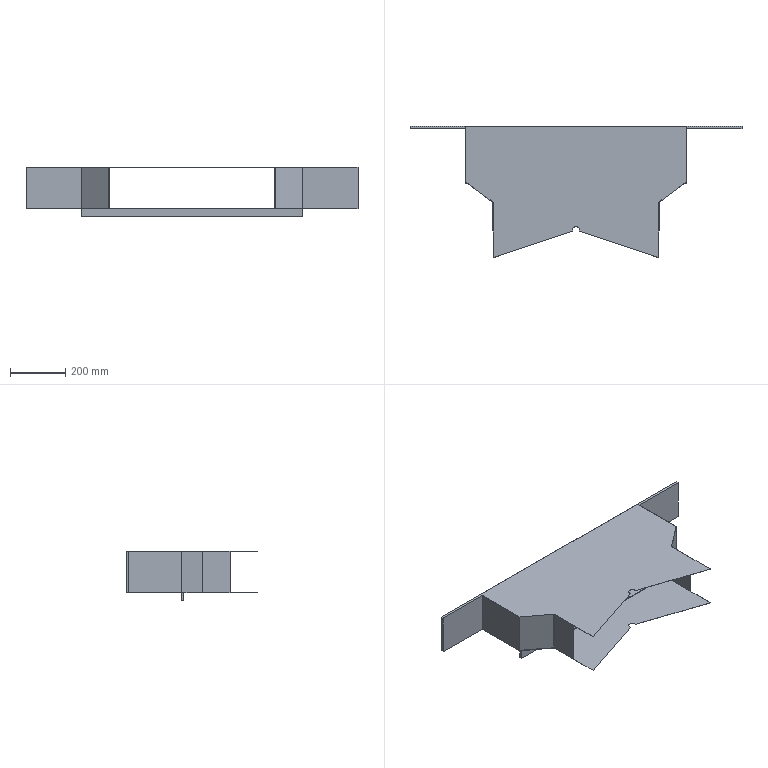Part | SolidWorks | features ICE 9, Extrusion 1 | 1 solid | 50 faces | box 1201 x 475 x 180 mm | volume 1092637 mm3 | plane 48 | cylinder 2 | commonest cylinder face diameters 25 x2
STEP:
#1=CARTESIAN_POINT('',(-399.925,274.7,0.));
#2=VERTEX_POINT('',#1);
#3=CARTESIAN_POINT('',(-399.598,274.7,0.));
#4=VERTEX_POINT('',#3);
#5=CARTESIAN_POINT('',(400.075,275.,0.));
#6=DIRECTION('',(1.,0.0003753,0.));
#7=VECTOR('',#6,1000.);
#8=LINE('',#5,#7);
#9=EDGE_CURVE('',#2,#4,#8,.T.);
#10=ORIENTED_EDGE('',*,*,#9,.F.);
#11=CARTESIAN_POINT('',(-399.925,274.195,0.));
#12=VERTEX_POINT('',#11);
#13=CARTESIAN_POINT('',(-399.922,266.7,0.));
#14=DIRECTION('',(-0.0003753,1.,0.));
#15=VECTOR('',#14,1000.);
#16=LINE('',#13,#15);
#17=EDGE_CURVE('',#12,#2,#16,.T.);
#18=ORIENTED_EDGE('',*,*,#17,.F.);
#19=CARTESIAN_POINT('',(-400.6,274.7,0.));
#20=VERTEX_POINT('',#19);
#21=CARTESIAN_POINT('',(-400.6,274.7,0.));
#22=DIRECTION('',(-0.8012,0.5985,0.));
#23=VECTOR('',#22,1000.);
#24=LINE('',#21,#23);
#25=EDGE_CURVE('',#12,#20,#24,.T.);
#26=ORIENTED_EDGE('',*,*,#25,.T.);
#27=CARTESIAN_POINT('',(-400.6,467.317,0.));
#28=VERTEX_POINT('',#27);
#29=CARTESIAN_POINT('',(-400.6,274.7,0.));
#30=DIRECTION('',(0.,1.,0.));
#31=VECTOR('',#30,1000.);
#32=LINE('',#29,#31);
#33=EDGE_CURVE('',#20,#28,#32,.T.);
#34=ORIENTED_EDGE('',*,*,#33,.T.);
#35=CARTESIAN_POINT('',(-600.6,467.317,0.));
#36=VERTEX_POINT('',#35);
#37=CARTESIAN_POINT('',(-600.6,467.317,0.));
#38=DIRECTION('',(1.,0.,0.));
#39=VECTOR('',#38,1000.);
#40=LINE('',#37,#39);
#41=EDGE_CURVE('',#36,#28,#40,.T.);
#42=ORIENTED_EDGE('',*,*,#41,.F.);
#43=CARTESIAN_POINT('',(-600.6,475.,0.));
#44=VERTEX_POINT('',#43);
#45=CARTESIAN_POINT('',(-600.6,467.317,0.));
#46=DIRECTION('',(0.,-1.,0.));
#47=VECTOR('',#46,1000.);
#48=LINE('',#45,#47);
#49=EDGE_CURVE('',#44,#36,#48,.T.);
#50=ORIENTED_EDGE('',*,*,#49,.F.);
#51=CARTESIAN_POINT('',(-400.,475.,0.));
#52=VERTEX_POINT('',#51);
#53=CARTESIAN_POINT('',(-400.6,475.,0.));
#54=DIRECTION('',(-1.,0.,0.));
#55=VECTOR('',#54,1000.);
#56=LINE('',#53,#55);
#57=EDGE_CURVE('',#52,#44,#56,.T.);
#58=ORIENTED_EDGE('',*,*,#57,.F.);
#59=CARTESIAN_POINT('',(-400.,275.,0.));
#60=VERTEX_POINT('',#59);
#61=CARTESIAN_POINT('',(-400.,375.,0.));
#62=DIRECTION('',(0.,-1.,0.));
#63=VECTOR('',#62,1000.);
#64=LINE('',#61,#63);
#65=EDGE_CURVE('',#52,#60,#64,.T.);
#66=ORIENTED_EDGE('',*,*,#65,.T.);
#67=CARTESIAN_POINT('',(-400.,275.,0.));
#68=DIRECTION('',(0.8012,-0.5985,0.));
#69=VECTOR('',#68,1000.);
#70=LINE('',#67,#69);
#71=EDGE_CURVE('',#60,#4,#70,.T.);
#72=ORIENTED_EDGE('',*,*,#71,.T.);
#73=EDGE_LOOP('',(#10,#18,#26,#34,#42,#50,#58,#66,#72));
#74=FACE_OUTER_BOUND('',#73,.T.);
#75=CARTESIAN_POINT('',(0.,100.,0.));
#76=DIRECTION('',(0.,0.,1.));
#77=DIRECTION('',(1.,0.,0.));
#78=AXIS2_PLACEMENT_3D('',#75,#76,#77);
#79=PLANE('',#78);
#80=ADVANCED_FACE('',(#74),#79,.F.);
#81=CARTESIAN_POINT('',(400.,275.,0.));
#82=VERTEX_POINT('',#81);
#83=CARTESIAN_POINT('',(400.075,275.,0.));
#84=VERTEX_POINT('',#83);
#85=CARTESIAN_POINT('',(400.075,275.,0.));
#86=DIRECTION('',(1.,0.0003753,0.));
#87=VECTOR('',#86,1000.);
#88=LINE('',#85,#87);
#89=EDGE_CURVE('',#82,#84,#88,.T.);
#90=ORIENTED_EDGE('',*,*,#89,.F.);
#91=CARTESIAN_POINT('',(400.,475.,0.));
#92=VERTEX_POINT('',#91);
#93=CARTESIAN_POINT('',(400.,375.,0.));
#94=DIRECTION('',(0.,1.,0.));
#95=VECTOR('',#94,1000.);
#96=LINE('',#93,#95);
#97=EDGE_CURVE('',#82,#92,#96,.T.);
#98=ORIENTED_EDGE('',*,*,#97,.T.);
#99=CARTESIAN_POINT('',(600.6,475.,0.));
#100=VERTEX_POINT('',#99);
#101=CARTESIAN_POINT('',(400.6,475.,0.));
#102=DIRECTION('',(-1.,0.,0.));
#103=VECTOR('',#102,1000.);
#104=LINE('',#101,#103);
#105=EDGE_CURVE('',#100,#92,#104,.T.);
#106=ORIENTED_EDGE('',*,*,#105,.F.);
#107=CARTESIAN_POINT('',(600.6,465.599,0.));
#108=VERTEX_POINT('',#107);
#109=CARTESIAN_POINT('',(600.6,475.,0.));
#110=DIRECTION('',(0.,1.,0.));
#111=VECTOR('',#110,1000.);
#112=LINE('',#109,#111);
#113=EDGE_CURVE('',#108,#100,#112,.T.);
#114=ORIENTED_EDGE('',*,*,#113,.F.);
#115=CARTESIAN_POINT('',(400.6,465.599,0.));
#116=VERTEX_POINT('',#115);
#117=CARTESIAN_POINT('',(600.6,465.599,0.));
#118=DIRECTION('',(-1.,0.,0.));
#119=VECTOR('',#118,1000.);
#120=LINE('',#117,#119);
#121=EDGE_CURVE('',#108,#116,#120,.T.);
#122=ORIENTED_EDGE('',*,*,#121,.T.);
#123=CARTESIAN_POINT('',(400.6,274.7,0.));
#124=VERTEX_POINT('',#123);
#125=CARTESIAN_POINT('',(400.6,274.7,0.));
#126=DIRECTION('',(0.,-1.,0.));
#127=VECTOR('',#126,1000.);
#128=LINE('',#125,#127);
#129=EDGE_CURVE('',#116,#124,#128,.T.);
#130=ORIENTED_EDGE('',*,*,#129,.T.);
#131=CARTESIAN_POINT('',(400.075,274.307,0.));
#132=VERTEX_POINT('',#131);
#133=CARTESIAN_POINT('',(400.6,274.7,0.));
#134=DIRECTION('',(-0.8012,-0.5985,0.));
#135=VECTOR('',#134,1000.);
#136=LINE('',#133,#135);
#137=EDGE_CURVE('',#124,#132,#136,.T.);
#138=ORIENTED_EDGE('',*,*,#137,.T.);
#139=CARTESIAN_POINT('',(400.078,267.,0.));
#140=DIRECTION('',(-0.0003753,1.,0.));
#141=VECTOR('',#140,1000.);
#142=LINE('',#139,#141);
#143=EDGE_CURVE('',#132,#84,#142,.T.);
#144=ORIENTED_EDGE('',*,*,#143,.T.);
#145=EDGE_LOOP('',(#90,#98,#106,#114,#122,#130,#138,#144));
#146=FACE_OUTER_BOUND('',#145,.T.);
#147=CARTESIAN_POINT('',(0.,100.,0.));
#148=DIRECTION('',(0.,0.,1.));
#149=DIRECTION('',(1.,0.,0.));
#150=AXIS2_PLACEMENT_3D('',#147,#148,#149);
#151=PLANE('',#150);
#152=ADVANCED_FACE('',(#146),#151,.F.);
#153=CARTESIAN_POINT('',(-300.,200.301,149.4));
#154=VERTEX_POINT('',#153);
#155=CARTESIAN_POINT('',(-300.,200.301,0.6));
#156=VERTEX_POINT('',#155);
#157=CARTESIAN_POINT('',(-300.,200.301,150.));
#158=DIRECTION('',(0.,0.,-1.));
#159=VECTOR('',#158,1000.);
#160=LINE('',#157,#159);
#161=EDGE_CURVE('',#154,#156,#160,.T.);
#162=ORIENTED_EDGE('',*,*,#161,.F.);
#163=CARTESIAN_POINT('',(-300.,100.,149.4));
#164=VERTEX_POINT('',#163);
#165=CARTESIAN_POINT('',(-300.,200.,149.4));
#166=DIRECTION('',(0.,-1.,0.));
#167=VECTOR('',#166,1000.);
#168=LINE('',#165,#167);
#169=EDGE_CURVE('',#154,#164,#168,.T.);
#170=ORIENTED_EDGE('',*,*,#169,.T.);
#171=CARTESIAN_POINT('',(-300.,100.,0.6));
#172=VERTEX_POINT('',#171);
#173=CARTESIAN_POINT('',(-300.,100.,150.));
#174=DIRECTION('',(0.,0.,-1.));
#175=VECTOR('',#174,1000.);
#176=LINE('',#173,#175);
#177=EDGE_CURVE('',#164,#172,#176,.T.);
#178=ORIENTED_EDGE('',*,*,#177,.T.);
#179=CARTESIAN_POINT('',(-300.,230.,0.6));
#180=DIRECTION('',(0.,-1.,0.));
#181=VECTOR('',#180,1000.);
#182=LINE('',#179,#181);
#183=EDGE_CURVE('',#156,#172,#182,.T.);
#184=ORIENTED_EDGE('',*,*,#183,.F.);
#185=EDGE_LOOP('',(#162,#170,#178,#184));
#186=FACE_OUTER_BOUND('',#185,.T.);
#187=CARTESIAN_POINT('',(-300.,200.,150.));
#188=DIRECTION('',(1.,0.,0.));
#189=DIRECTION('',(0.,0.,-1.));
#190=AXIS2_PLACEMENT_3D('',#187,#188,#189);
#191=PLANE('',#190);
#192=ADVANCED_FACE('',(#186),#191,.T.);
#193=CARTESIAN_POINT('',(-399.598,274.7,2.));
#194=VERTEX_POINT('',#193);
#195=CARTESIAN_POINT('',(-399.598,274.7,150.));
#196=DIRECTION('',(0.,0.,1.));
#197=VECTOR('',#196,1000.);
#198=LINE('',#195,#197);
#199=EDGE_CURVE('',#4,#194,#198,.T.);
#200=ORIENTED_EDGE('',*,*,#199,.F.);
#201=ORIENTED_EDGE('',*,*,#71,.F.);
#202=CARTESIAN_POINT('',(-400.,275.,149.4));
#203=VERTEX_POINT('',#202);
#204=CARTESIAN_POINT('',(-400.,275.,150.));
#205=DIRECTION('',(0.,0.,-1.));
#206=VECTOR('',#205,1000.);
#207=LINE('',#204,#206);
#208=EDGE_CURVE('',#203,#60,#207,.T.);
#209=ORIENTED_EDGE('',*,*,#208,.F.);
#210=CARTESIAN_POINT('',(-400.,275.,149.4));
#211=DIRECTION('',(0.8012,-0.5985,0.));
#212=VECTOR('',#211,1000.);
#213=LINE('',#210,#212);
#214=EDGE_CURVE('',#203,#154,#213,.T.);
#215=ORIENTED_EDGE('',*,*,#214,.T.);
#216=ORIENTED_EDGE('',*,*,#161,.T.);
#217=CARTESIAN_POINT('',(-342.578,232.106,0.6));
#218=VERTEX_POINT('',#217);
#219=CARTESIAN_POINT('',(-400.,275.,0.6));
#220=DIRECTION('',(0.8012,-0.5985,0.));
#221=VECTOR('',#220,1000.);
#222=LINE('',#219,#221);
#223=EDGE_CURVE('',#218,#156,#222,.T.);
#224=ORIENTED_EDGE('',*,*,#223,.F.);
#225=CARTESIAN_POINT('',(-342.578,232.106,2.));
#226=VERTEX_POINT('',#225);
#227=CARTESIAN_POINT('',(-342.578,232.106,2.));
#228=DIRECTION('',(0.,0.,-1.));
#229=VECTOR('',#228,1000.);
#230=LINE('',#227,#229);
#231=EDGE_CURVE('',#226,#218,#230,.T.);
#232=ORIENTED_EDGE('',*,*,#231,.F.);
#233=CARTESIAN_POINT('',(-400.,275.,2.));
#234=DIRECTION('',(0.8012,-0.5985,0.));
#235=VECTOR('',#234,1000.);
#236=LINE('',#233,#235);
#237=EDGE_CURVE('',#194,#226,#236,.T.);
#238=ORIENTED_EDGE('',*,*,#237,.F.);
#239=EDGE_LOOP('',(#200,#201,#209,#215,#216,#224,#232,#238));
#240=FACE_OUTER_BOUND('',#239,.T.);
#241=CARTESIAN_POINT('',(-400.,275.,150.));
#242=DIRECTION('',(0.5985,0.8012,0.));
#243=DIRECTION('',(-0.8012,0.5985,0.));
#244=AXIS2_PLACEMENT_3D('',#241,#242,#243);
#245=PLANE('',#244);
#246=ADVANCED_FACE('',(#240),#245,.T.);
#247=ORIENTED_EDGE('',*,*,#65,.F.);
#248=CARTESIAN_POINT('',(-400.,475.,149.4));
#249=VERTEX_POINT('',#248);
#250=CARTESIAN_POINT('',(-400.,475.,0.));
#251=DIRECTION('',(0.,0.,-1.));
#252=VECTOR('',#251,1000.);
#253=LINE('',#250,#252);
#254=EDGE_CURVE('',#249,#52,#253,.T.);
#255=ORIENTED_EDGE('',*,*,#254,.F.);
#256=CARTESIAN_POINT('',(-400.,375.,149.4));
#257=DIRECTION('',(0.,-1.,0.));
#258=VECTOR('',#257,1000.);
#259=LINE('',#256,#258);
#260=EDGE_CURVE('',#249,#203,#259,.T.);
#261=ORIENTED_EDGE('',*,*,#260,.T.);
#262=ORIENTED_EDGE('',*,*,#208,.T.);
#263=EDGE_LOOP('',(#247,#255,#261,#262));
#264=FACE_OUTER_BOUND('',#263,.T.);
#265=CARTESIAN_POINT('',(-400.,375.,150.));
#266=DIRECTION('',(1.,0.,0.));
#267=DIRECTION('',(0.,0.,-1.));
#268=AXIS2_PLACEMENT_3D('',#265,#266,#267);
#269=PLANE('',#268);
#270=ADVANCED_FACE('',(#264),#269,.T.);
#271=CARTESIAN_POINT('',(300.,100.,149.4));
#272=VERTEX_POINT('',#271);
#273=CARTESIAN_POINT('',(300.,100.,0.6));
#274=VERTEX_POINT('',#273);
#275=CARTESIAN_POINT('',(300.,100.,150.));
#276=DIRECTION('',(0.,0.,-1.));
#277=VECTOR('',#276,1000.);
#278=LINE('',#275,#277);
#279=EDGE_CURVE('',#272,#274,#278,.T.);
#280=ORIENTED_EDGE('',*,*,#279,.F.);
#281=CARTESIAN_POINT('',(300.,200.301,149.4));
#282=VERTEX_POINT('',#281);
#283=CARTESIAN_POINT('',(300.,200.,149.4));
#284=DIRECTION('',(0.,1.,0.));
#285=VECTOR('',#284,1000.);
#286=LINE('',#283,#285);
#287=EDGE_CURVE('',#272,#282,#286,.T.);
#288=ORIENTED_EDGE('',*,*,#287,.T.);
#289=CARTESIAN_POINT('',(300.,200.301,0.6));
#290=VERTEX_POINT('',#289);
#291=CARTESIAN_POINT('',(300.,200.301,150.));
#292=DIRECTION('',(0.,0.,-1.));
#293=VECTOR('',#292,1000.);
#294=LINE('',#291,#293);
#295=EDGE_CURVE('',#282,#290,#294,.T.);
#296=ORIENTED_EDGE('',*,*,#295,.T.);
#297=CARTESIAN_POINT('',(300.,0.,0.6));
#298=DIRECTION('',(0.,1.,0.));
#299=VECTOR('',#298,1000.);
#300=LINE('',#297,#299);
#301=EDGE_CURVE('',#274,#290,#300,.T.);
#302=ORIENTED_EDGE('',*,*,#301,.F.);
#303=EDGE_LOOP('',(#280,#288,#296,#302));
#304=FACE_OUTER_BOUND('',#303,.T.);
#305=CARTESIAN_POINT('',(300.,200.,150.));
#306=DIRECTION('',(-1.,0.,0.));
#307=DIRECTION('',(0.,0.,1.));
#308=AXIS2_PLACEMENT_3D('',#305,#306,#307);
#309=PLANE('',#308);
#310=ADVANCED_FACE('',(#304),#309,.T.);
#311=CARTESIAN_POINT('',(400.,275.,149.4));
#312=VERTEX_POINT('',#311);
#313=CARTESIAN_POINT('',(400.,275.,2.));
#314=VERTEX_POINT('',#313);
#315=CARTESIAN_POINT('',(400.,275.,150.));
#316=DIRECTION('',(0.,0.,-1.));
#317=VECTOR('',#316,1000.);
#318=LINE('',#315,#317);
#319=EDGE_CURVE('',#312,#314,#318,.T.);
#320=ORIENTED_EDGE('',*,*,#319,.F.);
#321=CARTESIAN_POINT('',(400.,475.,149.4));
#322=VERTEX_POINT('',#321);
#323=CARTESIAN_POINT('',(400.,375.,149.4));
#324=DIRECTION('',(0.,1.,0.));
#325=VECTOR('',#324,1000.);
#326=LINE('',#323,#325);
#327=EDGE_CURVE('',#312,#322,#326,.T.);
#328=ORIENTED_EDGE('',*,*,#327,.T.);
#329=CARTESIAN_POINT('',(400.,475.,149.4));
#330=DIRECTION('',(0.,0.,1.));
#331=VECTOR('',#330,1000.);
#332=LINE('',#329,#331);
#333=EDGE_CURVE('',#92,#322,#332,.T.);
#334=ORIENTED_EDGE('',*,*,#333,.F.);
#335=ORIENTED_EDGE('',*,*,#97,.F.);
#336=CARTESIAN_POINT('',(400.,275.,2.));
#337=DIRECTION('',(0.,0.,-1.));
#338=VECTOR('',#337,1000.);
#339=LINE('',#336,#338);
#340=EDGE_CURVE('',#314,#82,#339,.T.);
#341=ORIENTED_EDGE('',*,*,#340,.F.);
#342=EDGE_LOOP('',(#320,#328,#334,#335,#341));
#343=FACE_OUTER_BOUND('',#342,.T.);
#344=CARTESIAN_POINT('',(400.,375.,150.));
#345=DIRECTION('',(-1.,0.,0.));
#346=DIRECTION('',(0.,0.,1.));
#347=AXIS2_PLACEMENT_3D('',#344,#345,#346);
#348=PLANE('',#347);
#349=ADVANCED_FACE('',(#343),#348,.T.);
#350=CARTESIAN_POINT('',(339.758,230.,2.));
#351=VERTEX_POINT('',#350);
#352=CARTESIAN_POINT('',(339.758,230.,0.6));
#353=VERTEX_POINT('',#352);
#354=CARTESIAN_POINT('',(339.758,230.,2.));
#355=DIRECTION('',(0.,0.,-1.));
#356=VECTOR('',#355,1000.);
#357=LINE('',#354,#356);
#358=EDGE_CURVE('',#351,#353,#357,.T.);
#359=ORIENTED_EDGE('',*,*,#358,.T.);
#360=CARTESIAN_POINT('',(400.,275.,0.6));
#361=DIRECTION('',(-0.8012,-0.5985,0.));
#362=VECTOR('',#361,1000.);
#363=LINE('',#360,#362);
#364=EDGE_CURVE('',#353,#290,#363,.T.);
#365=ORIENTED_EDGE('',*,*,#364,.T.);
#366=ORIENTED_EDGE('',*,*,#295,.F.);
#367=CARTESIAN_POINT('',(400.,275.,149.4));
#368=DIRECTION('',(0.8012,0.5985,0.));
#369=VECTOR('',#368,1000.);
#370=LINE('',#367,#369);
#371=EDGE_CURVE('',#282,#312,#370,.T.);
#372=ORIENTED_EDGE('',*,*,#371,.T.);
#373=ORIENTED_EDGE('',*,*,#319,.T.);
#374=CARTESIAN_POINT('',(339.758,230.,2.));
#375=DIRECTION('',(-0.8012,-0.5985,0.));
#376=VECTOR('',#375,1000.);
#377=LINE('',#374,#376);
#378=EDGE_CURVE('',#314,#351,#377,.T.);
#379=ORIENTED_EDGE('',*,*,#378,.T.);
#380=EDGE_LOOP('',(#359,#365,#366,#372,#373,#379));
#381=FACE_OUTER_BOUND('',#380,.T.);
#382=CARTESIAN_POINT('',(400.,275.,150.));
#383=DIRECTION('',(-0.5985,0.8012,0.));
#384=DIRECTION('',(-0.8012,-0.5985,0.));
#385=AXIS2_PLACEMENT_3D('',#382,#383,#384);
#386=PLANE('',#385);
#387=ADVANCED_FACE('',(#381),#386,.T.);
#388=CARTESIAN_POINT('',(300.,100.,0.));
#389=VERTEX_POINT('',#388);
#390=CARTESIAN_POINT('',(300.,100.,150.));
#391=DIRECTION('',(0.,0.,-1.));
#392=VECTOR('',#391,1000.);
#393=LINE('',#390,#392);
#394=EDGE_CURVE('',#274,#389,#393,.T.);
#395=ORIENTED_EDGE('',*,*,#394,.F.);
#396=CARTESIAN_POINT('',(300.,0.,0.6));
#397=VERTEX_POINT('',#396);
#398=CARTESIAN_POINT('',(300.,0.,0.6));
#399=DIRECTION('',(0.,1.,0.));
#400=VECTOR('',#399,1000.);
#401=LINE('',#398,#400);
#402=EDGE_CURVE('',#397,#274,#401,.T.);
#403=ORIENTED_EDGE('',*,*,#402,.F.);
#404=CARTESIAN_POINT('',(300.,0.,0.));
#405=VERTEX_POINT('',#404);
#406=CARTESIAN_POINT('',(300.,0.,0.6));
#407=DIRECTION('',(0.,0.,-1.));
#408=VECTOR('',#407,1000.);
#409=LINE('',#406,#408);
#410=EDGE_CURVE('',#397,#405,#409,.T.);
#411=ORIENTED_EDGE('',*,*,#410,.T.);
#412=CARTESIAN_POINT('',(300.,0.,0.));
#413=DIRECTION('',(0.,1.,0.));
#414=VECTOR('',#413,1000.);
#415=LINE('',#412,#414);
#416=EDGE_CURVE('',#405,#389,#415,.T.);
#417=ORIENTED_EDGE('',*,*,#416,.T.);
#418=EDGE_LOOP('',(#395,#403,#411,#417));
#419=FACE_OUTER_BOUND('',#418,.T.);
#420=CARTESIAN_POINT('',(300.,0.,0.6));
#421=DIRECTION('',(-1.,0.,0.));
#422=DIRECTION('',(0.,0.,1.));
#423=AXIS2_PLACEMENT_3D('',#420,#421,#422);
#424=PLANE('',#423);
#425=ADVANCED_FACE('',(#419),#424,.F.);
#426=CARTESIAN_POINT('',(12.5,95.833,0.6));
#427=VERTEX_POINT('',#426);
#428=CARTESIAN_POINT('',(9.487,96.838,0.6));
#429=DIRECTION('',(0.9487,-0.3162,0.));
#430=VECTOR('',#429,1000.);
#431=LINE('',#428,#430);
#432=EDGE_CURVE('',#427,#397,#431,.T.);
#433=ORIENTED_EDGE('',*,*,#432,.F.);
#434=CARTESIAN_POINT('',(12.5,95.833,0.));
#435=VERTEX_POINT('',#434);
#436=CARTESIAN_POINT('',(12.5,95.833,0.6));
#437=DIRECTION('',(0.,0.,-1.));
#438=VECTOR('',#437,1000.);
#439=LINE('',#436,#438);
#440=EDGE_CURVE('',#427,#435,#439,.T.);
#441=ORIENTED_EDGE('',*,*,#440,.T.);
#442=CARTESIAN_POINT('',(9.487,96.838,0.));
#443=DIRECTION('',(0.9487,-0.3162,0.));
#444=VECTOR('',#443,1000.);
#445=LINE('',#442,#444);
#446=EDGE_CURVE('',#435,#405,#445,.T.);
#447=ORIENTED_EDGE('',*,*,#446,.T.);
#448=ORIENTED_EDGE('',*,*,#410,.F.);
#449=EDGE_LOOP('',(#433,#441,#447,#448));
#450=FACE_OUTER_BOUND('',#449,.T.);
#451=CARTESIAN_POINT('',(9.487,96.838,0.6));
#452=DIRECTION('',(0.3162,0.9487,0.));
#453=DIRECTION('',(-0.9487,0.3162,0.));
#454=AXIS2_PLACEMENT_3D('',#451,#452,#453);
#455=PLANE('',#454);
#456=ADVANCED_FACE('',(#450),#455,.F.);
#457=CARTESIAN_POINT('',(339.758,230.,0.));
#458=VERTEX_POINT('',#457);
#459=CARTESIAN_POINT('',(-300.,230.,0.));
#460=VERTEX_POINT('',#459);
#461=CARTESIAN_POINT('',(300.,230.,0.));
#462=DIRECTION('',(-1.,0.,0.));
#463=VECTOR('',#462,1000.);
#464=LINE('',#461,#463);
#465=EDGE_CURVE('',#458,#460,#464,.T.);
#466=ORIENTED_EDGE('',*,*,#465,.T.);
#467=CARTESIAN_POINT('',(-300.,230.,0.6));
#468=VERTEX_POINT('',#467);
#469=CARTESIAN_POINT('',(-300.,230.,0.6));
#470=DIRECTION('',(0.,0.,-1.));
#471=VECTOR('',#470,1000.);
#472=LINE('',#469,#471);
#473=EDGE_CURVE('',#468,#460,#472,.T.);
#474=ORIENTED_EDGE('',*,*,#473,.F.);
#475=CARTESIAN_POINT('',(300.,230.,0.6));
#476=DIRECTION('',(-1.,0.,0.));
#477=VECTOR('',#476,1000.);
#478=LINE('',#475,#477);
#479=EDGE_CURVE('',#353,#468,#478,.T.);
#480=ORIENTED_EDGE('',*,*,#479,.F.);
#481=CARTESIAN_POINT('',(339.758,230.,150.));
#482=DIRECTION('',(0.,0.,-1.));
#483=VECTOR('',#482,1000.);
#484=LINE('',#481,#483);
#485=EDGE_CURVE('',#353,#458,#484,.T.);
#486=ORIENTED_EDGE('',*,*,#485,.T.);
#487=EDGE_LOOP('',(#466,#474,#480,#486));
#488=FACE_OUTER_BOUND('',#487,.T.);
#489=CARTESIAN_POINT('',(300.,230.,0.6));
#490=DIRECTION('',(0.,-1.,0.));
#491=DIRECTION('',(1.,0.,0.));
#492=AXIS2_PLACEMENT_3D('',#489,#490,#491);
#493=PLANE('',#492);
#494=ADVANCED_FACE('',(#488),#493,.F.);
#495=CARTESIAN_POINT('',(-300.,0.,0.6));
#496=VERTEX_POINT('',#495);
#497=CARTESIAN_POINT('',(-300.,230.,0.6));
#498=DIRECTION('',(0.,-1.,0.));
#499=VECTOR('',#498,1000.);
#500=LINE('',#497,#499);
#501=EDGE_CURVE('',#172,#496,#500,.T.);
#502=ORIENTED_EDGE('',*,*,#501,.F.);
#503=CARTESIAN_POINT('',(-300.,100.,0.));
#504=VERTEX_POINT('',#503);
#505=CARTESIAN_POINT('',(-300.,100.,150.));
#506=DIRECTION('',(0.,0.,-1.));
#507=VECTOR('',#506,1000.);
#508=LINE('',#505,#507);
#509=EDGE_CURVE('',#172,#504,#508,.T.);
#510=ORIENTED_EDGE('',*,*,#509,.T.);
#511=CARTESIAN_POINT('',(-300.,0.,0.));
#512=VERTEX_POINT('',#511);
#513=CARTESIAN_POINT('',(-300.,230.,0.));
#514=DIRECTION('',(0.,-1.,0.));
#515=VECTOR('',#514,1000.);
#516=LINE('',#513,#515);
#517=EDGE_CURVE('',#504,#512,#516,.T.);
#518=ORIENTED_EDGE('',*,*,#517,.T.);
#519=CARTESIAN_POINT('',(-300.,0.,0.6));
#520=DIRECTION('',(0.,0.,-1.));
#521=VECTOR('',#520,1000.);
#522=LINE('',#519,#521);
#523=EDGE_CURVE('',#496,#512,#522,.T.);
#524=ORIENTED_EDGE('',*,*,#523,.F.);
#525=EDGE_LOOP('',(#502,#510,#518,#524));
#526=FACE_OUTER_BOUND('',#525,.T.);
#527=CARTESIAN_POINT('',(-300.,230.,0.6));
#528=DIRECTION('',(1.,0.,0.));
#529=DIRECTION('',(0.,1.,0.));
#530=AXIS2_PLACEMENT_3D('',#527,#528,#529);
#531=PLANE('',#530);
#532=ADVANCED_FACE('',(#526),#531,.F.);
#533=CARTESIAN_POINT('',(-12.5,95.833,0.));
#534=VERTEX_POINT('',#533);
#535=CARTESIAN_POINT('',(-9.487,96.838,0.));
#536=DIRECTION('',(0.9487,0.3162,0.));
#537=VECTOR('',#536,1000.);
#538=LINE('',#535,#537);
#539=EDGE_CURVE('',#512,#534,#538,.T.);
#540=ORIENTED_EDGE('',*,*,#539,.T.);
#541=CARTESIAN_POINT('',(-12.5,95.833,0.6));
#542=VERTEX_POINT('',#541);
#543=CARTESIAN_POINT('',(-12.5,95.833,0.6));
#544=DIRECTION('',(0.,0.,1.));
#545=VECTOR('',#544,1000.);
#546=LINE('',#543,#545);
#547=EDGE_CURVE('',#534,#542,#546,.T.);
#548=ORIENTED_EDGE('',*,*,#547,.T.);
#549=CARTESIAN_POINT('',(-9.487,96.838,0.6));
#550=DIRECTION('',(0.9487,0.3162,0.));
#551=VECTOR('',#550,1000.);
#552=LINE('',#549,#551);
#553=EDGE_CURVE('',#496,#542,#552,.T.);
#554=ORIENTED_EDGE('',*,*,#553,.F.);
#555=ORIENTED_EDGE('',*,*,#523,.T.);
#556=EDGE_LOOP('',(#540,#548,#554,#555));
#557=FACE_OUTER_BOUND('',#556,.T.);
#558=CARTESIAN_POINT('',(-9.487,96.838,0.6));
#559=DIRECTION('',(-0.3162,0.9487,0.));
#560=DIRECTION('',(-0.9487,-0.3162,0.));
#561=AXIS2_PLACEMENT_3D('',#558,#559,#560);
#562=PLANE('',#561);
#563=ADVANCED_FACE('',(#557),#562,.F.);
#564=CARTESIAN_POINT('',(12.5,100.,0.6));
#565=VERTEX_POINT('',#564);
#566=CARTESIAN_POINT('',(12.5,100.,0.6));
#567=DIRECTION('',(0.,1.,0.));
#568=VECTOR('',#567,1000.);
#569=LINE('',#566,#568);
#570=EDGE_CURVE('',#427,#565,#569,.T.);
#571=ORIENTED_EDGE('',*,*,#570,.F.);
#572=ORIENTED_EDGE('',*,*,#432,.T.);
#573=ORIENTED_EDGE('',*,*,#402,.T.);
#574=ORIENTED_EDGE('',*,*,#301,.T.);
#575=ORIENTED_EDGE('',*,*,#364,.F.);
#576=ORIENTED_EDGE('',*,*,#479,.T.);
#577=CARTESIAN_POINT('',(-300.,230.,0.6));
#578=DIRECTION('',(0.9988,-0.04941,0.));
#579=VECTOR('',#578,1000.);
#580=LINE('',#577,#579);
#581=EDGE_CURVE('',#218,#468,#580,.T.);
#582=ORIENTED_EDGE('',*,*,#581,.F.);
#583=ORIENTED_EDGE('',*,*,#223,.T.);
#584=ORIENTED_EDGE('',*,*,#183,.T.);
#585=ORIENTED_EDGE('',*,*,#501,.T.);
#586=ORIENTED_EDGE('',*,*,#553,.T.);
#587=CARTESIAN_POINT('',(-12.5,100.,0.6));
#588=VERTEX_POINT('',#587);
#589=CARTESIAN_POINT('',(-12.5,100.,0.6));
#590=DIRECTION('',(0.,-1.,0.));
#591=VECTOR('',#590,1000.);
#592=LINE('',#589,#591);
#593=EDGE_CURVE('',#588,#542,#592,.T.);
#594=ORIENTED_EDGE('',*,*,#593,.F.);
#595=CARTESIAN_POINT('',(0.,100.,0.6));
#596=DIRECTION('',(0.,0.,1.));
#597=DIRECTION('',(1.,0.,0.));
#598=AXIS2_PLACEMENT_3D('',#595,#596,#597);
#599=CIRCLE('',#598,12.5);
#600=EDGE_CURVE('',#565,#588,#599,.T.);
#601=ORIENTED_EDGE('',*,*,#600,.F.);
#602=EDGE_LOOP('',(#571,#572,#573,#574,#575,#576,#582,#583,#584,#585,#586,#594,#601));
#603=FACE_OUTER_BOUND('',#602,.T.);
#604=CARTESIAN_POINT('',(0.,100.,0.6));
#605=DIRECTION('',(0.,0.,1.));
#606=DIRECTION('',(1.,0.,0.));
#607=AXIS2_PLACEMENT_3D('',#604,#605,#606);
#608=PLANE('',#607);
#609=ADVANCED_FACE('',(#603),#608,.T.);
#610=CARTESIAN_POINT('',(-342.578,232.106,0.));
#611=VERTEX_POINT('',#610);
#612=CARTESIAN_POINT('',(-342.578,232.106,0.));
#613=DIRECTION('',(-1.,0.003087,0.));
#614=VECTOR('',#613,1000.);
#615=LINE('',#612,#614);
#616=EDGE_CURVE('',#458,#611,#615,.T.);
#617=ORIENTED_EDGE('',*,*,#616,.T.);
#618=CARTESIAN_POINT('',(-300.,230.,0.));
#619=DIRECTION('',(0.9988,-0.04941,0.));
#620=VECTOR('',#619,1000.);
#621=LINE('',#618,#620);
#622=EDGE_CURVE('',#611,#460,#621,.T.);
#623=ORIENTED_EDGE('',*,*,#622,.T.);
#624=ORIENTED_EDGE('',*,*,#465,.F.);
#625=EDGE_LOOP('',(#617,#623,#624));
#626=FACE_BOUND('',#625,.T.);
#627=CARTESIAN_POINT('',(-300.6,200.,0.));
#628=VERTEX_POINT('',#627);
#629=CARTESIAN_POINT('',(-389.896,266.704,0.));
#630=VERTEX_POINT('',#629);
#631=CARTESIAN_POINT('',(-400.6,274.7,0.));
#632=DIRECTION('',(-0.8012,0.5985,0.));
#633=VECTOR('',#632,1000.);
#634=LINE('',#631,#633);
#635=EDGE_CURVE('',#628,#630,#634,.T.);
#636=ORIENTED_EDGE('',*,*,#635,.T.);
#637=CARTESIAN_POINT('',(390.288,266.996,0.));
#638=VERTEX_POINT('',#637);
#639=CARTESIAN_POINT('',(400.078,267.,0.));
#640=DIRECTION('',(1.,0.0003753,0.));
#641=VECTOR('',#640,1000.);
#642=LINE('',#639,#641);
#643=EDGE_CURVE('',#630,#638,#642,.T.);
#644=ORIENTED_EDGE('',*,*,#643,.T.);
#645=CARTESIAN_POINT('',(300.6,200.,0.));
#646=VERTEX_POINT('',#645);
#647=CARTESIAN_POINT('',(400.6,274.7,0.));
#648=DIRECTION('',(-0.8012,-0.5985,0.));
#649=VECTOR('',#648,1000.);
#650=LINE('',#647,#649);
#651=EDGE_CURVE('',#638,#646,#650,.T.);
#652=ORIENTED_EDGE('',*,*,#651,.T.);
#653=CARTESIAN_POINT('',(300.6,100.,0.));
#654=VERTEX_POINT('',#653);
#655=CARTESIAN_POINT('',(300.6,100.,0.));
#656=DIRECTION('',(0.,-1.,0.));
#657=VECTOR('',#656,1000.);
#658=LINE('',#655,#657);
#659=EDGE_CURVE('',#646,#654,#658,.T.);
#660=ORIENTED_EDGE('',*,*,#659,.T.);
#661=CARTESIAN_POINT('',(300.,100.,0.));
#662=DIRECTION('',(-1.,0.,0.));
#663=VECTOR('',#662,1000.);
#664=LINE('',#661,#663);
#665=EDGE_CURVE('',#654,#389,#664,.T.);
#666=ORIENTED_EDGE('',*,*,#665,.T.);
#667=ORIENTED_EDGE('',*,*,#416,.F.);
#668=ORIENTED_EDGE('',*,*,#446,.F.);
#669=CARTESIAN_POINT('',(12.5,100.,0.));
#670=VERTEX_POINT('',#669);
#671=CARTESIAN_POINT('',(12.5,100.,0.));
#672=DIRECTION('',(0.,1.,0.));
#673=VECTOR('',#672,1000.);
#674=LINE('',#671,#673);
#675=EDGE_CURVE('',#435,#670,#674,.T.);
#676=ORIENTED_EDGE('',*,*,#675,.T.);
#677=CARTESIAN_POINT('',(-12.5,100.,0.));
#678=VERTEX_POINT('',#677);
#679=CARTESIAN_POINT('',(0.,100.,0.));
#680=DIRECTION('',(0.,0.,1.));
#681=DIRECTION('',(1.,0.,0.));
#682=AXIS2_PLACEMENT_3D('',#679,#680,#681);
#683=CIRCLE('',#682,12.5);
#684=EDGE_CURVE('',#670,#678,#683,.T.);
#685=ORIENTED_EDGE('',*,*,#684,.T.);
#686=CARTESIAN_POINT('',(-12.5,100.,0.));
#687=DIRECTION('',(0.,-1.,0.));
#688=VECTOR('',#687,1000.);
#689=LINE('',#686,#688);
#690=EDGE_CURVE('',#678,#534,#689,.T.);
#691=ORIENTED_EDGE('',*,*,#690,.T.);
#692=ORIENTED_EDGE('',*,*,#539,.F.);
#693=ORIENTED_EDGE('',*,*,#517,.F.);
#694=CARTESIAN_POINT('',(-300.6,100.,0.));
#695=VERTEX_POINT('',#694);
#696=CARTESIAN_POINT('',(-300.,100.,0.));
#697=DIRECTION('',(-1.,0.,0.));
#698=VECTOR('',#697,1000.);
#699=LINE('',#696,#698);
#700=EDGE_CURVE('',#504,#695,#699,.T.);
#701=ORIENTED_EDGE('',*,*,#700,.T.);
#702=CARTESIAN_POINT('',(-300.6,100.,0.));
#703=DIRECTION('',(0.,1.,0.));
#704=VECTOR('',#703,1000.);
#705=LINE('',#702,#704);
#706=EDGE_CURVE('',#695,#628,#705,.T.);
#707=ORIENTED_EDGE('',*,*,#706,.T.);
#708=EDGE_LOOP('',(#636,#644,#652,#660,#666,#667,#668,#676,#685,#691,#692,#693,#701,#707));
#709=FACE_OUTER_BOUND('',#708,.T.);
#710=CARTESIAN_POINT('',(0.,100.,0.));
#711=DIRECTION('',(0.,0.,1.));
#712=DIRECTION('',(1.,0.,0.));
#713=AXIS2_PLACEMENT_3D('',#710,#711,#712);
#714=PLANE('',#713);
#715=ADVANCED_FACE('',(#626,#709),#714,.F.);
#716=CARTESIAN_POINT('',(-400.6,467.317,150.));
#717=VERTEX_POINT('',#716);
#718=CARTESIAN_POINT('',(-400.6,467.317,150.));
#719=DIRECTION('',(0.,0.,1.));
#720=VECTOR('',#719,1000.);
#721=LINE('',#718,#720);
#722=EDGE_CURVE('',#28,#717,#721,.T.);
#723=ORIENTED_EDGE('',*,*,#722,.F.);
#724=ORIENTED_EDGE('',*,*,#33,.F.);
#725=CARTESIAN_POINT('',(-400.6,274.7,150.));
#726=VERTEX_POINT('',#725);
#727=CARTESIAN_POINT('',(-400.6,274.7,150.));
#728=DIRECTION('',(0.,0.,-1.));
#729=VECTOR('',#728,1000.);
#730=LINE('',#727,#729);
#731=EDGE_CURVE('',#726,#20,#730,.T.);
#732=ORIENTED_EDGE('',*,*,#731,.F.);
#733=CARTESIAN_POINT('',(-400.6,274.7,150.));
#734=DIRECTION('',(0.,1.,0.));
#735=VECTOR('',#734,1000.);
#736=LINE('',#733,#735);
#737=EDGE_CURVE('',#726,#717,#736,.T.);
#738=ORIENTED_EDGE('',*,*,#737,.T.);
#739=EDGE_LOOP('',(#723,#724,#732,#738));
#740=FACE_OUTER_BOUND('',#739,.T.);
#741=CARTESIAN_POINT('',(-400.6,274.7,150.));
#742=DIRECTION('',(-1.,0.,0.));
#743=DIRECTION('',(0.,0.,1.));
#744=AXIS2_PLACEMENT_3D('',#741,#742,#743);
#745=PLANE('',#744);
#746=ADVANCED_FACE('',(#740),#745,.T.);
#747=ORIENTED_EDGE('',*,*,#731,.T.);
#748=ORIENTED_EDGE('',*,*,#25,.F.);
#749=CARTESIAN_POINT('',(-400.6,274.7,0.));
#750=DIRECTION('',(-0.8012,0.5985,0.));
#751=VECTOR('',#750,1000.);
#752=LINE('',#749,#751);
#753=EDGE_CURVE('',#630,#12,#752,.T.);
#754=ORIENTED_EDGE('',*,*,#753,.F.);
#755=ORIENTED_EDGE('',*,*,#635,.F.);
#756=CARTESIAN_POINT('',(-300.6,200.,150.));
#757=VERTEX_POINT('',#756);
#758=CARTESIAN_POINT('',(-300.6,200.,150.));
#759=DIRECTION('',(0.,0.,-1.));
#760=VECTOR('',#759,1000.);
#761=LINE('',#758,#760);
#762=EDGE_CURVE('',#757,#628,#761,.T.);
#763=ORIENTED_EDGE('',*,*,#762,.F.);
#764=CARTESIAN_POINT('',(-400.6,274.7,150.));
#765=DIRECTION('',(-0.8012,0.5985,0.));
#766=VECTOR('',#765,1000.);
#767=LINE('',#764,#766);
#768=EDGE_CURVE('',#757,#726,#767,.T.);
#769=ORIENTED_EDGE('',*,*,#768,.T.);
#770=EDGE_LOOP('',(#747,#748,#754,#755,#763,#769));
#771=FACE_OUTER_BOUND('',#770,.T.);
#772=CARTESIAN_POINT('',(-400.6,274.7,150.));
#773=DIRECTION('',(-0.5985,-0.8012,0.));
#774=DIRECTION('',(0.8012,-0.5985,0.));
#775=AXIS2_PLACEMENT_3D('',#772,#773,#774);
#776=PLANE('',#775);
#777=ADVANCED_FACE('',(#771),#776,.T.);
#778=ORIENTED_EDGE('',*,*,#762,.T.);
#779=ORIENTED_EDGE('',*,*,#706,.F.);
#780=CARTESIAN_POINT('',(-300.6,100.,150.));
#781=VERTEX_POINT('',#780);
#782=CARTESIAN_POINT('',(-300.6,100.,150.));
#783=DIRECTION('',(0.,0.,-1.));
#784=VECTOR('',#783,1000.);
#785=LINE('',#782,#784);
#786=EDGE_CURVE('',#781,#695,#785,.T.);
#787=ORIENTED_EDGE('',*,*,#786,.F.);
#788=CARTESIAN_POINT('',(-300.6,100.,150.));
#789=DIRECTION('',(0.,1.,0.));
#790=VECTOR('',#789,1000.);
#791=LINE('',#788,#790);
#792=EDGE_CURVE('',#781,#757,#791,.T.);
#793=ORIENTED_EDGE('',*,*,#792,.T.);
#794=EDGE_LOOP('',(#778,#779,#787,#793));
#795=FACE_OUTER_BOUND('',#794,.T.);
#796=CARTESIAN_POINT('',(-300.6,100.,150.));
#797=DIRECTION('',(-1.,0.,0.));
#798=DIRECTION('',(0.,-1.,0.));
#799=AXIS2_PLACEMENT_3D('',#796,#797,#798);
#800=PLANE('',#799);
#801=ADVANCED_FACE('',(#795),#800,.T.);
#802=ORIENTED_EDGE('',*,*,#786,.T.);
#803=ORIENTED_EDGE('',*,*,#700,.F.);
#804=ORIENTED_EDGE('',*,*,#509,.F.);
#805=ORIENTED_EDGE('',*,*,#177,.F.);
#806=CARTESIAN_POINT('',(-300.,100.,150.));
#807=VERTEX_POINT('',#806);
#808=CARTESIAN_POINT('',(-300.,100.,150.));
#809=DIRECTION('',(0.,0.,-1.));
#810=VECTOR('',#809,1000.);
#811=LINE('',#808,#810);
#812=EDGE_CURVE('',#807,#164,#811,.T.);
#813=ORIENTED_EDGE('',*,*,#812,.F.);
#814=CARTESIAN_POINT('',(-300.,100.,150.));
#815=DIRECTION('',(-1.,0.,0.));
#816=VECTOR('',#815,1000.);
#817=LINE('',#814,#816);
#818=EDGE_CURVE('',#807,#781,#817,.T.);
#819=ORIENTED_EDGE('',*,*,#818,.T.);
#820=EDGE_LOOP('',(#802,#803,#804,#805,#813,#819));
#821=FACE_OUTER_BOUND('',#820,.T.);
#822=CARTESIAN_POINT('',(-300.,100.,150.));
#823=DIRECTION('',(0.,-1.,0.));
#824=DIRECTION('',(0.,0.,-1.));
#825=AXIS2_PLACEMENT_3D('',#822,#823,#824);
#826=PLANE('',#825);
#827=ADVANCED_FACE('',(#821),#826,.T.);
#828=CARTESIAN_POINT('',(12.5,100.,150.));
#829=VERTEX_POINT('',#828);
#830=CARTESIAN_POINT('',(-12.5,100.,150.));
#831=VERTEX_POINT('',#830);
#832=CARTESIAN_POINT('',(0.,100.,150.));
#833=DIRECTION('',(0.,0.,1.));
#834=DIRECTION('',(1.,0.,0.));
#835=AXIS2_PLACEMENT_3D('',#832,#833,#834);
#836=CIRCLE('',#835,12.5);
#837=EDGE_CURVE('',#829,#831,#836,.T.);
#838=ORIENTED_EDGE('',*,*,#837,.F.);
#839=CARTESIAN_POINT('',(12.5,95.833,150.));
#840=VERTEX_POINT('',#839);
#841=CARTESIAN_POINT('',(12.5,86.104,150.));
#842=DIRECTION('',(0.,1.,0.));
#843=VECTOR('',#842,1000.);
#844=LINE('',#841,#843);
#845=EDGE_CURVE('',#840,#829,#844,.T.);
#846=ORIENTED_EDGE('',*,*,#845,.F.);
#847=CARTESIAN_POINT('',(300.,0.,150.));
#848=VERTEX_POINT('',#847);
#849=CARTESIAN_POINT('',(300.,0.,150.));
#850=DIRECTION('',(0.9487,-0.3162,0.));
#851=VECTOR('',#850,1000.);
#852=LINE('',#849,#851);
#853=EDGE_CURVE('',#840,#848,#852,.T.);
#854=ORIENTED_EDGE('',*,*,#853,.T.);
#855=CARTESIAN_POINT('',(300.,100.,150.));
#856=VERTEX_POINT('',#855);
#857=CARTESIAN_POINT('',(300.,115.,150.));
#858=DIRECTION('',(0.,1.,0.));
#859=VECTOR('',#858,1000.);
#860=LINE('',#857,#859);
#861=EDGE_CURVE('',#848,#856,#860,.T.);
#862=ORIENTED_EDGE('',*,*,#861,.T.);
#863=CARTESIAN_POINT('',(300.6,100.,150.));
#864=VERTEX_POINT('',#863);
#865=CARTESIAN_POINT('',(300.,100.,150.));
#866=DIRECTION('',(-1.,0.,0.));
#867=VECTOR('',#866,1000.);
#868=LINE('',#865,#867);
#869=EDGE_CURVE('',#864,#856,#868,.T.);
#870=ORIENTED_EDGE('',*,*,#869,.F.);
#871=CARTESIAN_POINT('',(300.6,200.,150.));
#872=VERTEX_POINT('',#871);
#873=CARTESIAN_POINT('',(300.6,100.,150.));
#874=DIRECTION('',(0.,-1.,0.));
#875=VECTOR('',#874,1000.);
#876=LINE('',#873,#875);
#877=EDGE_CURVE('',#872,#864,#876,.T.);
#878=ORIENTED_EDGE('',*,*,#877,.F.);
#879=CARTESIAN_POINT('',(400.6,274.7,150.));
#880=VERTEX_POINT('',#879);
#881=CARTESIAN_POINT('',(400.6,274.7,150.));
#882=DIRECTION('',(-0.8012,-0.5985,0.));
#883=VECTOR('',#882,1000.);
#884=LINE('',#881,#883);
#885=EDGE_CURVE('',#880,#872,#884,.T.);
#886=ORIENTED_EDGE('',*,*,#885,.F.);
#887=CARTESIAN_POINT('',(400.6,465.599,150.));
#888=VERTEX_POINT('',#887);
#889=CARTESIAN_POINT('',(400.6,274.7,150.));
#890=DIRECTION('',(0.,-1.,0.));
#891=VECTOR('',#890,1000.);
#892=LINE('',#889,#891);
#893=EDGE_CURVE('',#888,#880,#892,.T.);
#894=ORIENTED_EDGE('',*,*,#893,.F.);
#895=CARTESIAN_POINT('',(600.6,465.599,150.));
#896=VERTEX_POINT('',#895);
#897=CARTESIAN_POINT('',(600.6,465.599,150.));
#898=DIRECTION('',(-1.,0.,0.));
#899=VECTOR('',#898,1000.);
#900=LINE('',#897,#899);
#901=EDGE_CURVE('',#896,#888,#900,.T.);
#902=ORIENTED_EDGE('',*,*,#901,.F.);
#903=CARTESIAN_POINT('',(600.6,475.,150.));
#904=VERTEX_POINT('',#903);
#905=CARTESIAN_POINT('',(600.6,465.599,150.));
#906=DIRECTION('',(0.,-1.,0.));
#907=VECTOR('',#906,1000.);
#908=LINE('',#905,#907);
#909=EDGE_CURVE('',#904,#896,#908,.T.);
#910=ORIENTED_EDGE('',*,*,#909,.F.);
#911=CARTESIAN_POINT('',(-600.6,475.,150.));
#912=VERTEX_POINT('',#911);
#913=CARTESIAN_POINT('',(-400.6,475.,150.));
#914=DIRECTION('',(1.,0.,0.));
#915=VECTOR('',#914,1000.);
#916=LINE('',#913,#915);
#917=EDGE_CURVE('',#912,#904,#916,.T.);
#918=ORIENTED_EDGE('',*,*,#917,.F.);
#919=CARTESIAN_POINT('',(-600.6,467.317,150.));
#920=VERTEX_POINT('',#919);
#921=CARTESIAN_POINT('',(-600.6,475.,150.));
#922=DIRECTION('',(0.,1.,0.));
#923=VECTOR('',#922,1000.);
#924=LINE('',#921,#923);
#925=EDGE_CURVE('',#920,#912,#924,.T.);
#926=ORIENTED_EDGE('',*,*,#925,.F.);
#927=CARTESIAN_POINT('',(-600.6,467.317,150.));
#928=DIRECTION('',(1.,0.,0.));
#929=VECTOR('',#928,1000.);
#930=LINE('',#927,#929);
#931=EDGE_CURVE('',#920,#717,#930,.T.);
#932=ORIENTED_EDGE('',*,*,#931,.T.);
#933=ORIENTED_EDGE('',*,*,#737,.F.);
#934=ORIENTED_EDGE('',*,*,#768,.F.);
#935=ORIENTED_EDGE('',*,*,#792,.F.);
#936=ORIENTED_EDGE('',*,*,#818,.F.);
#937=CARTESIAN_POINT('',(-300.,0.,150.));
#938=VERTEX_POINT('',#937);
#939=CARTESIAN_POINT('',(-300.,0.,150.));
#940=DIRECTION('',(0.,-1.,0.));
#941=VECTOR('',#940,1000.);
#942=LINE('',#939,#941);
#943=EDGE_CURVE('',#807,#938,#942,.T.);
#944=ORIENTED_EDGE('',*,*,#943,.T.);
#945=CARTESIAN_POINT('',(-12.5,95.833,150.));
#946=VERTEX_POINT('',#945);
#947=CARTESIAN_POINT('',(-9.487,96.838,150.));
#948=DIRECTION('',(0.9487,0.3162,0.));
#949=VECTOR('',#948,1000.);
#950=LINE('',#947,#949);
#951=EDGE_CURVE('',#938,#946,#950,.T.);
#952=ORIENTED_EDGE('',*,*,#951,.T.);
#953=CARTESIAN_POINT('',(-12.5,100.,150.));
#954=DIRECTION('',(0.,-1.,0.));
#955=VECTOR('',#954,1000.);
#956=LINE('',#953,#955);
#957=EDGE_CURVE('',#831,#946,#956,.T.);
#958=ORIENTED_EDGE('',*,*,#957,.F.);
#959=EDGE_LOOP('',(#838,#846,#854,#862,#870,#878,#886,#894,#902,#910,#918,#926,#932,#933,#934,#935,#936,#944,#952,#958));
#960=FACE_OUTER_BOUND('',#959,.T.);
#961=CARTESIAN_POINT('',(0.,0.,150.));
#962=DIRECTION('',(0.,0.,-1.));
#963=DIRECTION('',(-1.,0.,0.));
#964=AXIS2_PLACEMENT_3D('',#961,#962,#963);
#965=PLANE('',#964);
#966=ADVANCED_FACE('',(#960),#965,.F.);
#967=ORIENTED_EDGE('',*,*,#665,.F.);
#968=CARTESIAN_POINT('',(300.6,100.,150.));
#969=DIRECTION('',(0.,0.,-1.));
#970=VECTOR('',#969,1000.);
#971=LINE('',#968,#970);
#972=EDGE_CURVE('',#864,#654,#971,.T.);
#973=ORIENTED_EDGE('',*,*,#972,.F.);
#974=ORIENTED_EDGE('',*,*,#869,.T.);
#975=CARTESIAN_POINT('',(300.,100.,150.));
#976=DIRECTION('',(0.,0.,-1.));
#977=VECTOR('',#976,1000.);
#978=LINE('',#975,#977);
#979=EDGE_CURVE('',#856,#272,#978,.T.);
#980=ORIENTED_EDGE('',*,*,#979,.T.);
#981=ORIENTED_EDGE('',*,*,#279,.T.);
#982=ORIENTED_EDGE('',*,*,#394,.T.);
#983=EDGE_LOOP('',(#967,#973,#974,#980,#981,#982));
#984=FACE_OUTER_BOUND('',#983,.T.);
#985=CARTESIAN_POINT('',(300.,100.,150.));
#986=DIRECTION('',(0.,-1.,0.));
#987=DIRECTION('',(0.,0.,-1.));
#988=AXIS2_PLACEMENT_3D('',#985,#986,#987);
#989=PLANE('',#988);
#990=ADVANCED_FACE('',(#984),#989,.T.);
#991=ORIENTED_EDGE('',*,*,#877,.T.);
#992=ORIENTED_EDGE('',*,*,#972,.T.);
#993=ORIENTED_EDGE('',*,*,#659,.F.);
#994=CARTESIAN_POINT('',(300.6,200.,150.));
#995=DIRECTION('',(0.,0.,-1.));
#996=VECTOR('',#995,1000.);
#997=LINE('',#994,#996);
#998=EDGE_CURVE('',#872,#646,#997,.T.);
#999=ORIENTED_EDGE('',*,*,#998,.F.);
#1000=EDGE_LOOP('',(#991,#992,#993,#999));
#1001=FACE_OUTER_BOUND('',#1000,.T.);
#1002=CARTESIAN_POINT('',(300.6,100.,150.));
#1003=DIRECTION('',(1.,0.,0.));
#1004=DIRECTION('',(0.,1.,0.));
#1005=AXIS2_PLACEMENT_3D('',#1002,#1003,#1004);
#1006=PLANE('',#1005);
#1007=ADVANCED_FACE('',(#1001),#1006,.T.);
#1008=ORIENTED_EDGE('',*,*,#998,.T.);
#1009=ORIENTED_EDGE('',*,*,#651,.F.);
#1010=CARTESIAN_POINT('',(400.6,274.7,0.));
#1011=DIRECTION('',(-0.8012,-0.5985,0.));
#1012=VECTOR('',#1011,1000.);
#1013=LINE('',#1010,#1012);
#1014=EDGE_CURVE('',#132,#638,#1013,.T.);
#1015=ORIENTED_EDGE('',*,*,#1014,.F.);
#1016=ORIENTED_EDGE('',*,*,#137,.F.);
#1017=CARTESIAN_POINT('',(400.6,274.7,150.));
#1018=DIRECTION('',(0.,0.,-1.));
#1019=VECTOR('',#1018,1000.);
#1020=LINE('',#1017,#1019);
#1021=EDGE_CURVE('',#880,#124,#1020,.T.);
#1022=ORIENTED_EDGE('',*,*,#1021,.F.);
#1023=ORIENTED_EDGE('',*,*,#885,.T.);
#1024=EDGE_LOOP('',(#1008,#1009,#1015,#1016,#1022,#1023));
#1025=FACE_OUTER_BOUND('',#1024,.T.);
#1026=CARTESIAN_POINT('',(400.6,274.7,150.));
#1027=DIRECTION('',(0.5985,-0.8012,0.));
#1028=DIRECTION('',(0.8012,0.5985,0.));
#1029=AXIS2_PLACEMENT_3D('',#1026,#1027,#1028);
#1030=PLANE('',#1029);
#1031=ADVANCED_FACE('',(#1025),#1030,.T.);
#1032=CARTESIAN_POINT('',(400.6,465.599,0.));
#1033=DIRECTION('',(0.,0.,-1.));
#1034=VECTOR('',#1033,1000.);
#1035=LINE('',#1032,#1034);
#1036=EDGE_CURVE('',#888,#116,#1035,.T.);
#1037=ORIENTED_EDGE('',*,*,#1036,.F.);
#1038=ORIENTED_EDGE('',*,*,#893,.T.);
#1039=ORIENTED_EDGE('',*,*,#1021,.T.);
#1040=ORIENTED_EDGE('',*,*,#129,.F.);
#1041=EDGE_LOOP('',(#1037,#1038,#1039,#1040));
#1042=FACE_OUTER_BOUND('',#1041,.T.);
#1043=CARTESIAN_POINT('',(400.6,274.7,150.));
#1044=DIRECTION('',(1.,0.,0.));
#1045=DIRECTION('',(0.,0.,-1.));
#1046=AXIS2_PLACEMENT_3D('',#1043,#1044,#1045);
#1047=PLANE('',#1046);
#1048=ADVANCED_FACE('',(#1042),#1047,.T.);
#1049=CARTESIAN_POINT('',(-12.5,95.833,149.4));
#1050=VERTEX_POINT('',#1049);
#1051=CARTESIAN_POINT('',(-12.5,95.833,149.4));
#1052=DIRECTION('',(0.,0.,-1.));
#1053=VECTOR('',#1052,1000.);
#1054=LINE('',#1051,#1053);
#1055=EDGE_CURVE('',#946,#1050,#1054,.T.);
#1056=ORIENTED_EDGE('',*,*,#1055,.F.);
#1057=ORIENTED_EDGE('',*,*,#951,.F.);
#1058=CARTESIAN_POINT('',(-300.,0.,149.4));
#1059=VERTEX_POINT('',#1058);
#1060=CARTESIAN_POINT('',(-300.,0.,149.4));
#1061=DIRECTION('',(0.,0.,1.));
#1062=VECTOR('',#1061,1000.);
#1063=LINE('',#1060,#1062);
#1064=EDGE_CURVE('',#1059,#938,#1063,.T.);
#1065=ORIENTED_EDGE('',*,*,#1064,.F.);
#1066=CARTESIAN_POINT('',(-9.487,96.838,149.4));
#1067=DIRECTION('',(0.9487,0.3162,0.));
#1068=VECTOR('',#1067,1000.);
#1069=LINE('',#1066,#1068);
#1070=EDGE_CURVE('',#1059,#1050,#1069,.T.);
#1071=ORIENTED_EDGE('',*,*,#1070,.T.);
#1072=EDGE_LOOP('',(#1056,#1057,#1065,#1071));
#1073=FACE_OUTER_BOUND('',#1072,.T.);
#1074=CARTESIAN_POINT('',(-9.487,96.838,149.4));
#1075=DIRECTION('',(0.3162,-0.9487,0.));
#1076=DIRECTION('',(0.9487,0.3162,0.));
#1077=AXIS2_PLACEMENT_3D('',#1074,#1075,#1076);
#1078=PLANE('',#1077);
#1079=ADVANCED_FACE('',(#1073),#1078,.T.);
#1080=ORIENTED_EDGE('',*,*,#943,.F.);
#1081=ORIENTED_EDGE('',*,*,#812,.T.);
#1082=CARTESIAN_POINT('',(-300.,0.,149.4));
#1083=DIRECTION('',(0.,-1.,0.));
#1084=VECTOR('',#1083,1000.);
#1085=LINE('',#1082,#1084);
#1086=EDGE_CURVE('',#164,#1059,#1085,.T.);
#1087=ORIENTED_EDGE('',*,*,#1086,.T.);
#1088=ORIENTED_EDGE('',*,*,#1064,.T.);
#1089=EDGE_LOOP('',(#1080,#1081,#1087,#1088));
#1090=FACE_OUTER_BOUND('',#1089,.T.);
#1091=CARTESIAN_POINT('',(-300.,0.,149.4));
#1092=DIRECTION('',(-1.,0.,0.));
#1093=DIRECTION('',(0.,-1.,0.));
#1094=AXIS2_PLACEMENT_3D('',#1091,#1092,#1093);
#1095=PLANE('',#1094);
#1096=ADVANCED_FACE('',(#1090),#1095,.T.);
#1097=CARTESIAN_POINT('',(300.,0.,149.4));
#1098=VERTEX_POINT('',#1097);
#1099=CARTESIAN_POINT('',(300.,115.,149.4));
#1100=DIRECTION('',(0.,1.,0.));
#1101=VECTOR('',#1100,1000.);
#1102=LINE('',#1099,#1101);
#1103=EDGE_CURVE('',#1098,#272,#1102,.T.);
#1104=ORIENTED_EDGE('',*,*,#1103,.T.);
#1105=ORIENTED_EDGE('',*,*,#979,.F.);
#1106=ORIENTED_EDGE('',*,*,#861,.F.);
#1107=CARTESIAN_POINT('',(300.,0.,149.4));
#1108=DIRECTION('',(0.,0.,1.));
#1109=VECTOR('',#1108,1000.);
#1110=LINE('',#1107,#1109);
#1111=EDGE_CURVE('',#1098,#848,#1110,.T.);
#1112=ORIENTED_EDGE('',*,*,#1111,.F.);
#1113=EDGE_LOOP('',(#1104,#1105,#1106,#1112));
#1114=FACE_OUTER_BOUND('',#1113,.T.);
#1115=CARTESIAN_POINT('',(300.,115.,149.4));
#1116=DIRECTION('',(1.,0.,0.));
#1117=DIRECTION('',(0.,0.,-1.));
#1118=AXIS2_PLACEMENT_3D('',#1115,#1116,#1117);
#1119=PLANE('',#1118);
#1120=ADVANCED_FACE('',(#1114),#1119,.T.);
#1121=CARTESIAN_POINT('',(12.5,95.833,149.4));
#1122=VERTEX_POINT('',#1121);
#1123=CARTESIAN_POINT('',(12.5,95.833,149.4));
#1124=DIRECTION('',(0.,0.,1.));
#1125=VECTOR('',#1124,1000.);
#1126=LINE('',#1123,#1125);
#1127=EDGE_CURVE('',#1122,#840,#1126,.T.);
#1128=ORIENTED_EDGE('',*,*,#1127,.F.);
#1129=CARTESIAN_POINT('',(300.,0.,149.4));
#1130=DIRECTION('',(0.9487,-0.3162,0.));
#1131=VECTOR('',#1130,1000.);
#1132=LINE('',#1129,#1131);
#1133=EDGE_CURVE('',#1122,#1098,#1132,.T.);
#1134=ORIENTED_EDGE('',*,*,#1133,.T.);
#1135=ORIENTED_EDGE('',*,*,#1111,.T.);
#1136=ORIENTED_EDGE('',*,*,#853,.F.);
#1137=EDGE_LOOP('',(#1128,#1134,#1135,#1136));
#1138=FACE_OUTER_BOUND('',#1137,.T.);
#1139=CARTESIAN_POINT('',(300.,0.,149.4));
#1140=DIRECTION('',(-0.3162,-0.9487,0.));
#1141=DIRECTION('',(0.9487,-0.3162,0.));
#1142=AXIS2_PLACEMENT_3D('',#1139,#1140,#1141);
#1143=PLANE('',#1142);
#1144=ADVANCED_FACE('',(#1138),#1143,.T.);
#1145=ORIENTED_EDGE('',*,*,#1133,.F.);
#1146=CARTESIAN_POINT('',(12.5,100.,149.4));
#1147=VERTEX_POINT('',#1146);
#1148=CARTESIAN_POINT('',(12.5,100.,149.4));
#1149=DIRECTION('',(0.,1.,0.));
#1150=VECTOR('',#1149,1000.);
#1151=LINE('',#1148,#1150);
#1152=EDGE_CURVE('',#1122,#1147,#1151,.T.);
#1153=ORIENTED_EDGE('',*,*,#1152,.T.);
#1154=CARTESIAN_POINT('',(-12.5,100.,149.4));
#1155=VERTEX_POINT('',#1154);
#1156=CARTESIAN_POINT('',(0.,100.,149.4));
#1157=DIRECTION('',(0.,0.,1.));
#1158=DIRECTION('',(1.,0.,0.));
#1159=AXIS2_PLACEMENT_3D('',#1156,#1157,#1158);
#1160=CIRCLE('',#1159,12.5);
#1161=EDGE_CURVE('',#1147,#1155,#1160,.T.);
#1162=ORIENTED_EDGE('',*,*,#1161,.T.);
#1163=CARTESIAN_POINT('',(-12.5,100.,149.4));
#1164=DIRECTION('',(0.,-1.,0.));
#1165=VECTOR('',#1164,1000.);
#1166=LINE('',#1163,#1165);
#1167=EDGE_CURVE('',#1155,#1050,#1166,.T.);
#1168=ORIENTED_EDGE('',*,*,#1167,.T.);
#1169=ORIENTED_EDGE('',*,*,#1070,.F.);
#1170=ORIENTED_EDGE('',*,*,#1086,.F.);
#1171=ORIENTED_EDGE('',*,*,#169,.F.);
#1172=ORIENTED_EDGE('',*,*,#214,.F.);
#1173=ORIENTED_EDGE('',*,*,#260,.F.);
#1174=CARTESIAN_POINT('',(-400.,475.,149.4));
#1175=DIRECTION('',(-1.,0.,0.));
#1176=VECTOR('',#1175,1000.);
#1177=LINE('',#1174,#1176);
#1178=EDGE_CURVE('',#322,#249,#1177,.T.);
#1179=ORIENTED_EDGE('',*,*,#1178,.F.);
#1180=ORIENTED_EDGE('',*,*,#327,.F.);
#1181=ORIENTED_EDGE('',*,*,#371,.F.);
#1182=ORIENTED_EDGE('',*,*,#287,.F.);
#1183=ORIENTED_EDGE('',*,*,#1103,.F.);
#1184=EDGE_LOOP('',(#1145,#1153,#1162,#1168,#1169,#1170,#1171,#1172,#1173,#1179,#1180,#1181,#1182,#1183));
#1185=FACE_OUTER_BOUND('',#1184,.T.);
#1186=CARTESIAN_POINT('',(0.,100.,149.4));
#1187=DIRECTION('',(0.,0.,1.));
#1188=DIRECTION('',(1.,0.,0.));
#1189=AXIS2_PLACEMENT_3D('',#1186,#1187,#1188);
#1190=PLANE('',#1189);
#1191=ADVANCED_FACE('',(#1185),#1190,.F.);
#1192=ORIENTED_EDGE('',*,*,#622,.F.);
#1193=CARTESIAN_POINT('',(-342.578,232.106,150.));
#1194=DIRECTION('',(0.,0.,1.));
#1195=VECTOR('',#1194,1000.);
#1196=LINE('',#1193,#1195);
#1197=EDGE_CURVE('',#611,#218,#1196,.T.);
#1198=ORIENTED_EDGE('',*,*,#1197,.T.);
#1199=ORIENTED_EDGE('',*,*,#581,.T.);
#1200=ORIENTED_EDGE('',*,*,#473,.T.);
#1201=EDGE_LOOP('',(#1192,#1198,#1199,#1200));
#1202=FACE_OUTER_BOUND('',#1201,.T.);
#1203=CARTESIAN_POINT('',(-300.,230.,0.6));
#1204=DIRECTION('',(0.04941,0.9988,0.));
#1205=DIRECTION('',(-0.9988,0.04941,0.));
#1206=AXIS2_PLACEMENT_3D('',#1203,#1204,#1205);
#1207=PLANE('',#1206);
#1208=ADVANCED_FACE('',(#1202),#1207,.T.);
#1209=ORIENTED_EDGE('',*,*,#1055,.T.);
#1210=ORIENTED_EDGE('',*,*,#1167,.F.);
#1211=CARTESIAN_POINT('',(-12.5,100.,-0.00005));
#1212=DIRECTION('',(0.,0.,1.));
#1213=VECTOR('',#1212,1000.);
#1214=LINE('',#1211,#1213);
#1215=EDGE_CURVE('',#1155,#831,#1214,.T.);
#1216=ORIENTED_EDGE('',*,*,#1215,.T.);
#1217=ORIENTED_EDGE('',*,*,#957,.T.);
#1218=EDGE_LOOP('',(#1209,#1210,#1216,#1217));
#1219=FACE_OUTER_BOUND('',#1218,.T.);
#1220=CARTESIAN_POINT('',(-12.5,100.,-0.00005));
#1221=DIRECTION('',(-1.,0.,0.));
#1222=DIRECTION('',(0.,0.,1.));
#1223=AXIS2_PLACEMENT_3D('',#1220,#1221,#1222);
#1224=PLANE('',#1223);
#1225=ADVANCED_FACE('',(#1219),#1224,.F.);
#1226=ORIENTED_EDGE('',*,*,#1127,.T.);
#1227=ORIENTED_EDGE('',*,*,#845,.T.);
#1228=CARTESIAN_POINT('',(12.5,100.,-0.00005));
#1229=DIRECTION('',(0.,0.,1.));
#1230=VECTOR('',#1229,1000.);
#1231=LINE('',#1228,#1230);
#1232=EDGE_CURVE('',#1147,#829,#1231,.T.);
#1233=ORIENTED_EDGE('',*,*,#1232,.F.);
#1234=ORIENTED_EDGE('',*,*,#1152,.F.);
#1235=EDGE_LOOP('',(#1226,#1227,#1233,#1234));
#1236=FACE_OUTER_BOUND('',#1235,.T.);
#1237=CARTESIAN_POINT('',(12.5,86.104,-0.00005));
#1238=DIRECTION('',(1.,0.,0.));
#1239=DIRECTION('',(0.,0.,-1.));
#1240=AXIS2_PLACEMENT_3D('',#1237,#1238,#1239);
#1241=PLANE('',#1240);
#1242=ADVANCED_FACE('',(#1236),#1241,.F.);
#1243=ORIENTED_EDGE('',*,*,#1232,.T.);
#1244=ORIENTED_EDGE('',*,*,#837,.T.);
#1245=ORIENTED_EDGE('',*,*,#1215,.F.);
#1246=ORIENTED_EDGE('',*,*,#1161,.F.);
#1247=EDGE_LOOP('',(#1243,#1244,#1245,#1246));
#1248=FACE_OUTER_BOUND('',#1247,.T.);
#1249=CARTESIAN_POINT('',(0.,100.,-0.00005));
#1250=DIRECTION('',(0.,0.,1.));
#1251=DIRECTION('',(1.,0.,0.));
#1252=AXIS2_PLACEMENT_3D('',#1249,#1250,#1251);
#1253=CYLINDRICAL_SURFACE('',#1252,12.5);
#1254=ADVANCED_FACE('',(#1248),#1253,.F.);
#1255=ORIENTED_EDGE('',*,*,#600,.T.);
#1256=CARTESIAN_POINT('',(-12.5,100.,-0.00005));
#1257=DIRECTION('',(0.,0.,1.));
#1258=VECTOR('',#1257,1000.);
#1259=LINE('',#1256,#1258);
#1260=EDGE_CURVE('',#678,#588,#1259,.T.);
#1261=ORIENTED_EDGE('',*,*,#1260,.F.);
#1262=ORIENTED_EDGE('',*,*,#684,.F.);
#1263=CARTESIAN_POINT('',(12.5,100.,-0.00005));
#1264=DIRECTION('',(0.,0.,1.));
#1265=VECTOR('',#1264,1000.);
#1266=LINE('',#1263,#1265);
#1267=EDGE_CURVE('',#670,#565,#1266,.T.);
#1268=ORIENTED_EDGE('',*,*,#1267,.T.);
#1269=EDGE_LOOP('',(#1255,#1261,#1262,#1268));
#1270=FACE_OUTER_BOUND('',#1269,.T.);
#1271=CARTESIAN_POINT('',(0.,100.,-0.00005));
#1272=DIRECTION('',(0.,0.,1.));
#1273=DIRECTION('',(1.,0.,0.));
#1274=AXIS2_PLACEMENT_3D('',#1271,#1272,#1273);
#1275=CYLINDRICAL_SURFACE('',#1274,12.5);
#1276=ADVANCED_FACE('',(#1270),#1275,.F.);
#1277=ORIENTED_EDGE('',*,*,#570,.T.);
#1278=ORIENTED_EDGE('',*,*,#1267,.F.);
#1279=ORIENTED_EDGE('',*,*,#675,.F.);
#1280=ORIENTED_EDGE('',*,*,#440,.F.);
#1281=EDGE_LOOP('',(#1277,#1278,#1279,#1280));
#1282=FACE_OUTER_BOUND('',#1281,.T.);
#1283=CARTESIAN_POINT('',(12.5,86.104,-0.00005));
#1284=DIRECTION('',(1.,0.,0.));
#1285=DIRECTION('',(0.,0.,-1.));
#1286=AXIS2_PLACEMENT_3D('',#1283,#1284,#1285);
#1287=PLANE('',#1286);
#1288=ADVANCED_FACE('',(#1282),#1287,.F.);
#1289=ORIENTED_EDGE('',*,*,#593,.T.);
#1290=ORIENTED_EDGE('',*,*,#547,.F.);
#1291=ORIENTED_EDGE('',*,*,#690,.F.);
#1292=ORIENTED_EDGE('',*,*,#1260,.T.);
#1293=EDGE_LOOP('',(#1289,#1290,#1291,#1292));
#1294=FACE_OUTER_BOUND('',#1293,.T.);
#1295=CARTESIAN_POINT('',(-12.5,100.,-0.00005));
#1296=DIRECTION('',(-1.,0.,0.));
#1297=DIRECTION('',(0.,0.,1.));
#1298=AXIS2_PLACEMENT_3D('',#1295,#1296,#1297);
#1299=PLANE('',#1298);
#1300=ADVANCED_FACE('',(#1294),#1299,.F.);
#1301=ORIENTED_EDGE('',*,*,#57,.T.);
#1302=CARTESIAN_POINT('',(-600.6,475.,0.));
#1303=DIRECTION('',(0.,0.,-1.));
#1304=VECTOR('',#1303,1000.);
#1305=LINE('',#1302,#1304);
#1306=EDGE_CURVE('',#912,#44,#1305,.T.);
#1307=ORIENTED_EDGE('',*,*,#1306,.F.);
#1308=ORIENTED_EDGE('',*,*,#917,.T.);
#1309=CARTESIAN_POINT('',(600.6,475.,150.));
#1310=DIRECTION('',(0.,0.,1.));
#1311=VECTOR('',#1310,1000.);
#1312=LINE('',#1309,#1311);
#1313=EDGE_CURVE('',#100,#904,#1312,.T.);
#1314=ORIENTED_EDGE('',*,*,#1313,.F.);
#1315=ORIENTED_EDGE('',*,*,#105,.T.);
#1316=ORIENTED_EDGE('',*,*,#333,.T.);
#1317=ORIENTED_EDGE('',*,*,#1178,.T.);
#1318=ORIENTED_EDGE('',*,*,#254,.T.);
#1319=EDGE_LOOP('',(#1301,#1307,#1308,#1314,#1315,#1316,#1317,#1318));
#1320=FACE_OUTER_BOUND('',#1319,.T.);
#1321=CARTESIAN_POINT('',(0.,475.,0.));
#1322=DIRECTION('',(0.,1.,0.));
#1323=DIRECTION('',(0.,0.,1.));
#1324=AXIS2_PLACEMENT_3D('',#1321,#1322,#1323);
#1325=PLANE('',#1324);
#1326=ADVANCED_FACE('',(#1320),#1325,.T.);
#1327=ORIENTED_EDGE('',*,*,#722,.T.);
#1328=ORIENTED_EDGE('',*,*,#931,.F.);
#1329=CARTESIAN_POINT('',(-600.6,467.317,150.));
#1330=DIRECTION('',(0.,0.,1.));
#1331=VECTOR('',#1330,1000.);
#1332=LINE('',#1329,#1331);
#1333=EDGE_CURVE('',#36,#920,#1332,.T.);
#1334=ORIENTED_EDGE('',*,*,#1333,.F.);
#1335=ORIENTED_EDGE('',*,*,#41,.T.);
#1336=EDGE_LOOP('',(#1327,#1328,#1334,#1335));
#1337=FACE_OUTER_BOUND('',#1336,.T.);
#1338=CARTESIAN_POINT('',(-600.6,467.317,150.));
#1339=DIRECTION('',(0.,1.,0.));
#1340=DIRECTION('',(0.,0.,1.));
#1341=AXIS2_PLACEMENT_3D('',#1338,#1339,#1340);
#1342=PLANE('',#1341);
#1343=ADVANCED_FACE('',(#1337),#1342,.F.);
#1344=ORIENTED_EDGE('',*,*,#49,.T.);
#1345=ORIENTED_EDGE('',*,*,#1333,.T.);
#1346=ORIENTED_EDGE('',*,*,#925,.T.);
#1347=ORIENTED_EDGE('',*,*,#1306,.T.);
#1348=EDGE_LOOP('',(#1344,#1345,#1346,#1347));
#1349=FACE_OUTER_BOUND('',#1348,.T.);
#1350=CARTESIAN_POINT('',(-600.6,0.,0.));
#1351=DIRECTION('',(1.,0.,0.));
#1352=DIRECTION('',(0.,0.,-1.));
#1353=AXIS2_PLACEMENT_3D('',#1350,#1351,#1352);
#1354=PLANE('',#1353);
#1355=ADVANCED_FACE('',(#1349),#1354,.F.);
#1356=ORIENTED_EDGE('',*,*,#1036,.T.);
#1357=ORIENTED_EDGE('',*,*,#121,.F.);
#1358=CARTESIAN_POINT('',(600.6,465.599,0.));
#1359=DIRECTION('',(0.,0.,-1.));
#1360=VECTOR('',#1359,1000.);
#1361=LINE('',#1358,#1360);
#1362=EDGE_CURVE('',#896,#108,#1361,.T.);
#1363=ORIENTED_EDGE('',*,*,#1362,.F.);
#1364=ORIENTED_EDGE('',*,*,#901,.T.);
#1365=EDGE_LOOP('',(#1356,#1357,#1363,#1364));
#1366=FACE_OUTER_BOUND('',#1365,.T.);
#1367=CARTESIAN_POINT('',(600.6,465.599,0.));
#1368=DIRECTION('',(0.,1.,0.));
#1369=DIRECTION('',(0.,0.,1.));
#1370=AXIS2_PLACEMENT_3D('',#1367,#1368,#1369);
#1371=PLANE('',#1370);
#1372=ADVANCED_FACE('',(#1366),#1371,.F.);
#1373=ORIENTED_EDGE('',*,*,#909,.T.);
#1374=ORIENTED_EDGE('',*,*,#1362,.T.);
#1375=ORIENTED_EDGE('',*,*,#113,.T.);
#1376=ORIENTED_EDGE('',*,*,#1313,.T.);
#1377=EDGE_LOOP('',(#1373,#1374,#1375,#1376));
#1378=FACE_OUTER_BOUND('',#1377,.T.);
#1379=CARTESIAN_POINT('',(600.6,0.,0.));
#1380=DIRECTION('',(-1.,0.,0.));
#1381=DIRECTION('',(0.,0.,1.));
#1382=AXIS2_PLACEMENT_3D('',#1379,#1380,#1381);
#1383=PLANE('',#1382);
#1384=ADVANCED_FACE('',(#1378),#1383,.F.);
#1385=ORIENTED_EDGE('',*,*,#616,.F.);
#1386=ORIENTED_EDGE('',*,*,#485,.F.);
#1387=ORIENTED_EDGE('',*,*,#358,.F.);
#1388=CARTESIAN_POINT('',(-342.578,232.106,2.));
#1389=DIRECTION('',(-1.,0.003087,0.));
#1390=VECTOR('',#1389,1000.);
#1391=LINE('',#1388,#1390);
#1392=EDGE_CURVE('',#351,#226,#1391,.T.);
#1393=ORIENTED_EDGE('',*,*,#1392,.T.);
#1394=ORIENTED_EDGE('',*,*,#231,.T.);
#1395=ORIENTED_EDGE('',*,*,#1197,.F.);
#1396=EDGE_LOOP('',(#1385,#1386,#1387,#1393,#1394,#1395));
#1397=FACE_OUTER_BOUND('',#1396,.T.);
#1398=CARTESIAN_POINT('',(-342.578,232.106,2.));
#1399=DIRECTION('',(-0.003087,-1.,0.));
#1400=DIRECTION('',(1.,-0.003087,0.));
#1401=AXIS2_PLACEMENT_3D('',#1398,#1399,#1400);
#1402=PLANE('',#1401);
#1403=ADVANCED_FACE('',(#1397),#1402,.T.);
#1404=ORIENTED_EDGE('',*,*,#340,.T.);
#1405=ORIENTED_EDGE('',*,*,#89,.T.);
#1406=CARTESIAN_POINT('',(400.075,275.,-30.));
#1407=VERTEX_POINT('',#1406);
#1408=CARTESIAN_POINT('',(400.075,275.,-30.));
#1409=DIRECTION('',(0.,0.,-1.));
#1410=VECTOR('',#1409,1000.);
#1411=LINE('',#1408,#1410);
#1412=EDGE_CURVE('',#84,#1407,#1411,.T.);
#1413=ORIENTED_EDGE('',*,*,#1412,.T.);
#1414=CARTESIAN_POINT('',(-399.925,274.7,-30.));
#1415=VERTEX_POINT('',#1414);
#1416=CARTESIAN_POINT('',(-399.925,274.7,-30.));
#1417=DIRECTION('',(-1.,-0.0003753,0.));
#1418=VECTOR('',#1417,1000.);
#1419=LINE('',#1416,#1418);
#1420=EDGE_CURVE('',#1407,#1415,#1419,.T.);
#1421=ORIENTED_EDGE('',*,*,#1420,.T.);
#1422=CARTESIAN_POINT('',(-399.925,274.7,0.));
#1423=DIRECTION('',(0.,0.,1.));
#1424=VECTOR('',#1423,1000.);
#1425=LINE('',#1422,#1424);
#1426=EDGE_CURVE('',#1415,#2,#1425,.T.);
#1427=ORIENTED_EDGE('',*,*,#1426,.T.);
#1428=ORIENTED_EDGE('',*,*,#9,.T.);
#1429=ORIENTED_EDGE('',*,*,#199,.T.);
#1430=CARTESIAN_POINT('',(400.,275.,2.));
#1431=DIRECTION('',(1.,0.0003753,0.));
#1432=VECTOR('',#1431,1000.);
#1433=LINE('',#1430,#1432);
#1434=EDGE_CURVE('',#194,#314,#1433,.T.);
#1435=ORIENTED_EDGE('',*,*,#1434,.T.);
#1436=EDGE_LOOP('',(#1404,#1405,#1413,#1421,#1427,#1428,#1429,#1435));
#1437=FACE_OUTER_BOUND('',#1436,.T.);
#1438=CARTESIAN_POINT('',(400.,275.,2.));
#1439=DIRECTION('',(-0.0003753,1.,0.));
#1440=DIRECTION('',(-1.,-0.0003753,0.));
#1441=AXIS2_PLACEMENT_3D('',#1438,#1439,#1440);
#1442=PLANE('',#1441);
#1443=ADVANCED_FACE('',(#1437),#1442,.T.);
#1444=ORIENTED_EDGE('',*,*,#1434,.F.);
#1445=ORIENTED_EDGE('',*,*,#237,.T.);
#1446=ORIENTED_EDGE('',*,*,#1392,.F.);
#1447=ORIENTED_EDGE('',*,*,#378,.F.);
#1448=EDGE_LOOP('',(#1444,#1445,#1446,#1447));
#1449=FACE_OUTER_BOUND('',#1448,.T.);
#1450=CARTESIAN_POINT('',(0.,0.,2.));
#1451=DIRECTION('',(0.,0.,1.));
#1452=DIRECTION('',(1.,0.,0.));
#1453=AXIS2_PLACEMENT_3D('',#1450,#1451,#1452);
#1454=PLANE('',#1453);
#1455=ADVANCED_FACE('',(#1449),#1454,.T.);
#1456=CARTESIAN_POINT('',(-399.922,266.7,0.));
#1457=VERTEX_POINT('',#1456);
#1458=CARTESIAN_POINT('',(400.078,267.,0.));
#1459=DIRECTION('',(1.,0.0003753,0.));
#1460=VECTOR('',#1459,1000.);
#1461=LINE('',#1458,#1460);
#1462=EDGE_CURVE('',#1457,#630,#1461,.T.);
#1463=ORIENTED_EDGE('',*,*,#1462,.T.);
#1464=ORIENTED_EDGE('',*,*,#753,.T.);
#1465=CARTESIAN_POINT('',(-399.922,266.7,0.));
#1466=DIRECTION('',(-0.0003753,1.,0.));
#1467=VECTOR('',#1466,1000.);
#1468=LINE('',#1465,#1467);
#1469=EDGE_CURVE('',#1457,#12,#1468,.T.);
#1470=ORIENTED_EDGE('',*,*,#1469,.F.);
#1471=EDGE_LOOP('',(#1463,#1464,#1470));
#1472=FACE_OUTER_BOUND('',#1471,.T.);
#1473=CARTESIAN_POINT('',(400.078,267.,0.));
#1474=DIRECTION('',(0.,0.,1.));
#1475=DIRECTION('',(1.,0.,0.));
#1476=AXIS2_PLACEMENT_3D('',#1473,#1474,#1475);
#1477=PLANE('',#1476);
#1478=ADVANCED_FACE('',(#1472),#1477,.T.);
#1479=CARTESIAN_POINT('',(400.078,267.,0.));
#1480=VERTEX_POINT('',#1479);
#1481=CARTESIAN_POINT('',(400.078,267.,0.));
#1482=DIRECTION('',(-0.0003753,1.,0.));
#1483=VECTOR('',#1482,1000.);
#1484=LINE('',#1481,#1483);
#1485=EDGE_CURVE('',#1480,#132,#1484,.T.);
#1486=ORIENTED_EDGE('',*,*,#1485,.T.);
#1487=ORIENTED_EDGE('',*,*,#1014,.T.);
#1488=CARTESIAN_POINT('',(400.078,267.,0.));
#1489=DIRECTION('',(1.,0.0003753,0.));
#1490=VECTOR('',#1489,1000.);
#1491=LINE('',#1488,#1490);
#1492=EDGE_CURVE('',#638,#1480,#1491,.T.);
#1493=ORIENTED_EDGE('',*,*,#1492,.T.);
#1494=EDGE_LOOP('',(#1486,#1487,#1493));
#1495=FACE_OUTER_BOUND('',#1494,.T.);
#1496=CARTESIAN_POINT('',(400.078,267.,0.));
#1497=DIRECTION('',(0.,0.,1.));
#1498=DIRECTION('',(1.,0.,0.));
#1499=AXIS2_PLACEMENT_3D('',#1496,#1497,#1498);
#1500=PLANE('',#1499);
#1501=ADVANCED_FACE('',(#1495),#1500,.T.);
#1502=ORIENTED_EDGE('',*,*,#1426,.F.);
#1503=CARTESIAN_POINT('',(-399.922,266.7,-30.));
#1504=VERTEX_POINT('',#1503);
#1505=CARTESIAN_POINT('',(-399.922,266.7,-30.));
#1506=DIRECTION('',(-0.0003753,1.,0.));
#1507=VECTOR('',#1506,1000.);
#1508=LINE('',#1505,#1507);
#1509=EDGE_CURVE('',#1504,#1415,#1508,.T.);
#1510=ORIENTED_EDGE('',*,*,#1509,.F.);
#1511=CARTESIAN_POINT('',(-399.922,266.7,0.));
#1512=DIRECTION('',(0.,0.,1.));
#1513=VECTOR('',#1512,1000.);
#1514=LINE('',#1511,#1513);
#1515=EDGE_CURVE('',#1504,#1457,#1514,.T.);
#1516=ORIENTED_EDGE('',*,*,#1515,.T.);
#1517=ORIENTED_EDGE('',*,*,#1469,.T.);
#1518=ORIENTED_EDGE('',*,*,#17,.T.);
#1519=EDGE_LOOP('',(#1502,#1510,#1516,#1517,#1518));
#1520=FACE_OUTER_BOUND('',#1519,.T.);
#1521=CARTESIAN_POINT('',(-399.922,266.7,0.));
#1522=DIRECTION('',(-1.,-0.0003753,0.));
#1523=DIRECTION('',(0.0003753,-1.,0.));
#1524=AXIS2_PLACEMENT_3D('',#1521,#1522,#1523);
#1525=PLANE('',#1524);
#1526=ADVANCED_FACE('',(#1520),#1525,.T.);
#1527=ORIENTED_EDGE('',*,*,#1420,.F.);
#1528=CARTESIAN_POINT('',(400.078,267.,-30.));
#1529=VERTEX_POINT('',#1528);
#1530=CARTESIAN_POINT('',(400.078,267.,-30.));
#1531=DIRECTION('',(-0.0003753,1.,0.));
#1532=VECTOR('',#1531,1000.);
#1533=LINE('',#1530,#1532);
#1534=EDGE_CURVE('',#1529,#1407,#1533,.T.);
#1535=ORIENTED_EDGE('',*,*,#1534,.F.);
#1536=CARTESIAN_POINT('',(-399.922,266.7,-30.));
#1537=DIRECTION('',(-1.,-0.0003753,0.));
#1538=VECTOR('',#1537,1000.);
#1539=LINE('',#1536,#1538);
#1540=EDGE_CURVE('',#1529,#1504,#1539,.T.);
#1541=ORIENTED_EDGE('',*,*,#1540,.T.);
#1542=ORIENTED_EDGE('',*,*,#1509,.T.);
#1543=EDGE_LOOP('',(#1527,#1535,#1541,#1542));
#1544=FACE_OUTER_BOUND('',#1543,.T.);
#1545=CARTESIAN_POINT('',(-399.922,266.7,-30.));
#1546=DIRECTION('',(0.,0.,-1.));
#1547=DIRECTION('',(-1.,0.,0.));
#1548=AXIS2_PLACEMENT_3D('',#1545,#1546,#1547);
#1549=PLANE('',#1548);
#1550=ADVANCED_FACE('',(#1544),#1549,.T.);
#1551=ORIENTED_EDGE('',*,*,#1412,.F.);
#1552=ORIENTED_EDGE('',*,*,#143,.F.);
#1553=ORIENTED_EDGE('',*,*,#1485,.F.);
#1554=CARTESIAN_POINT('',(400.078,267.,-30.));
#1555=DIRECTION('',(0.,0.,-1.));
#1556=VECTOR('',#1555,1000.);
#1557=LINE('',#1554,#1556);
#1558=EDGE_CURVE('',#1480,#1529,#1557,.T.);
#1559=ORIENTED_EDGE('',*,*,#1558,.T.);
#1560=ORIENTED_EDGE('',*,*,#1534,.T.);
#1561=EDGE_LOOP('',(#1551,#1552,#1553,#1559,#1560));
#1562=FACE_OUTER_BOUND('',#1561,.T.);
#1563=CARTESIAN_POINT('',(400.078,267.,-30.));
#1564=DIRECTION('',(1.,0.0003753,0.));
#1565=DIRECTION('',(-0.0003753,1.,0.));
#1566=AXIS2_PLACEMENT_3D('',#1563,#1564,#1565);
#1567=PLANE('',#1566);
#1568=ADVANCED_FACE('',(#1562),#1567,.T.);
#1569=ORIENTED_EDGE('',*,*,#1462,.F.);
#1570=ORIENTED_EDGE('',*,*,#1515,.F.);
#1571=ORIENTED_EDGE('',*,*,#1540,.F.);
#1572=ORIENTED_EDGE('',*,*,#1558,.F.);
#1573=ORIENTED_EDGE('',*,*,#1492,.F.);
#1574=ORIENTED_EDGE('',*,*,#643,.F.);
#1575=EDGE_LOOP('',(#1569,#1570,#1571,#1572,#1573,#1574));
#1576=FACE_OUTER_BOUND('',#1575,.T.);
#1577=CARTESIAN_POINT('',(-0.1001,266.85,0.));
#1578=DIRECTION('',(0.0003753,-1.,0.));
#1579=DIRECTION('',(1.,0.0003753,0.));
#1580=AXIS2_PLACEMENT_3D('',#1577,#1578,#1579);
#1581=PLANE('',#1580);
#1582=ADVANCED_FACE('',(#1576),#1581,.T.);
#1583=CLOSED_SHELL('',(#80,#152,#192,#246,#270,#310,#349,#387,#425,#456,#494,#532,#563,#609,#715,#746,#777,#801,#827,#966,#990,#1007,#1031,#1048,#1079,#1096,#1120,#1144,#1191,#1208,#1225,#1242,#1254,#1276,#1288,#1300,#1326,#1343,#1355,#1372,#1384,#1403,#1443,#1455,#1478,#1501,#1526,#1550,#1568,#1582));
#1584=MANIFOLD_SOLID_BREP('',#1583);
#1585=CARTESIAN_POINT('',(0.,0.,0.));
#1586=DIRECTION('',(0.,0.,1.));
#1587=DIRECTION('',(1.,0.,0.));
#1588=AXIS2_PLACEMENT_3D('',#1585,#1586,#1587);
#1589=(LENGTH_UNIT()NAMED_UNIT(*)SI_UNIT(.MILLI.,.METRE.));
#1590=UNCERTAINTY_MEASURE_WITH_UNIT(LENGTH_MEASURE(0.00001),#1589,'','');
#1591=(NAMED_UNIT(*)PLANE_ANGLE_UNIT()SI_UNIT($,.RADIAN.));
#1592=(NAMED_UNIT(*)SI_UNIT($,.STERADIAN.)SOLID_ANGLE_UNIT());
#1593=(GEOMETRIC_REPRESENTATION_CONTEXT(3)GLOBAL_UNCERTAINTY_ASSIGNED_CONTEXT((#1590))GLOBAL_UNIT_ASSIGNED_CONTEXT((#1589,#1591,#1592))REPRESENTATION_CONTEXT('',''));
#1594=ADVANCED_BREP_SHAPE_REPRESENTATION('',(#1584,#1588),#1593);